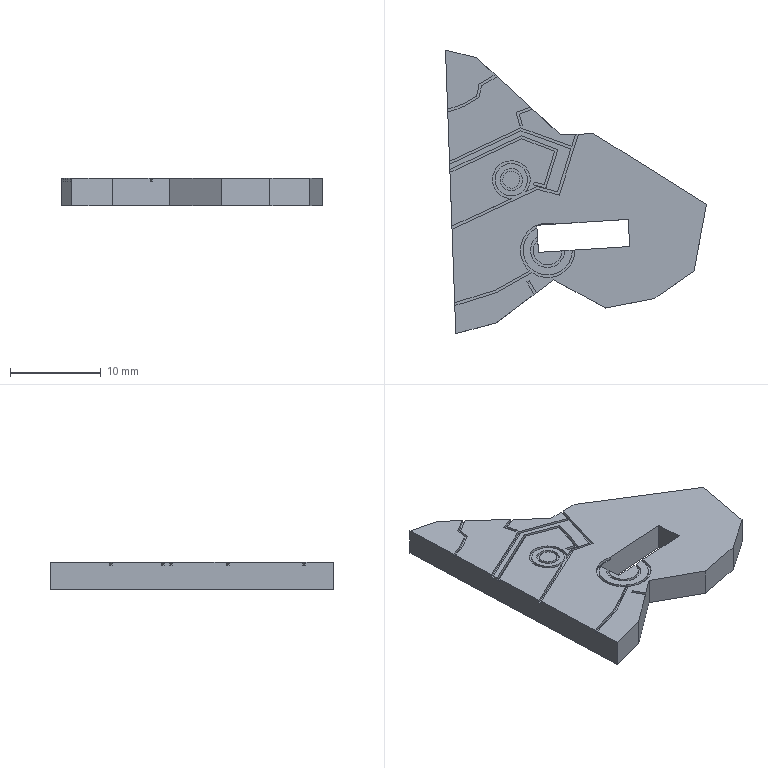Part | SolidWorks | features BaseBody 1 | 1 solid | 122 faces | box 28.758 x 31.242 x 3 mm | volume 1487 mm3 | plane 71 | spline 51